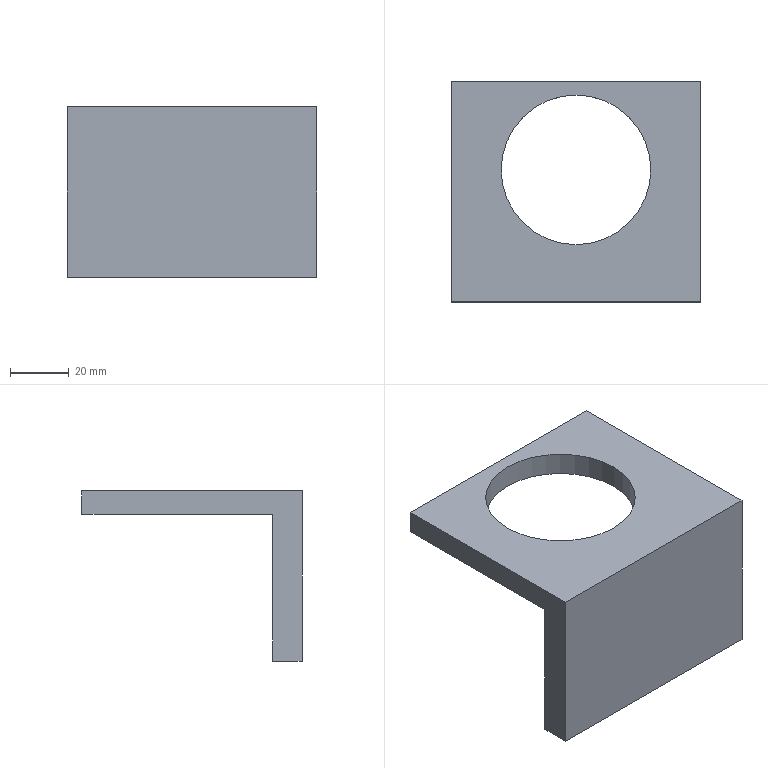Part | SolidWorks | features Extrusion 1, ICE 1 | 1 solid | 10 faces | box 85 x 75 x 58 mm | volume 77157 mm3 | plane 8 | cylinder 2 | commonest cylinder face diameters 51 x2
STEP:
#1=CARTESIAN_POINT('',(-25.5,0.,8.));
#2=VERTEX_POINT('',#1);
#3=CARTESIAN_POINT('',(25.5,0.,8.));
#4=VERTEX_POINT('',#3);
#5=CARTESIAN_POINT('',(0.,0.,8.));
#6=DIRECTION('',(0.,0.,1.));
#7=DIRECTION('',(1.,0.,0.));
#8=AXIS2_PLACEMENT_3D('',#5,#6,#7);
#9=CIRCLE('',#8,25.5);
#10=EDGE_CURVE('',#2,#4,#9,.T.);
#11=ORIENTED_EDGE('',*,*,#10,.T.);
#12=CARTESIAN_POINT('',(25.5,0.,0.));
#13=VERTEX_POINT('',#12);
#14=CARTESIAN_POINT('',(25.5,0.,8.));
#15=DIRECTION('',(0.,0.,-1.));
#16=VECTOR('',#15,1000.);
#17=LINE('',#14,#16);
#18=EDGE_CURVE('',#4,#13,#17,.T.);
#19=ORIENTED_EDGE('',*,*,#18,.T.);
#20=CARTESIAN_POINT('',(-25.5,0.,0.));
#21=VERTEX_POINT('',#20);
#22=CARTESIAN_POINT('',(0.,0.,0.));
#23=DIRECTION('',(0.,0.,1.));
#24=DIRECTION('',(1.,0.,0.));
#25=AXIS2_PLACEMENT_3D('',#22,#23,#24);
#26=CIRCLE('',#25,25.5);
#27=EDGE_CURVE('',#21,#13,#26,.T.);
#28=ORIENTED_EDGE('',*,*,#27,.F.);
#29=CARTESIAN_POINT('',(-25.5,0.,8.));
#30=DIRECTION('',(0.,0.,-1.));
#31=VECTOR('',#30,1000.);
#32=LINE('',#29,#31);
#33=EDGE_CURVE('',#2,#21,#32,.T.);
#34=ORIENTED_EDGE('',*,*,#33,.F.);
#35=EDGE_LOOP('',(#11,#19,#28,#34));
#36=FACE_OUTER_BOUND('',#35,.T.);
#37=CARTESIAN_POINT('',(0.,0.,8.));
#38=DIRECTION('',(0.,0.,-1.));
#39=DIRECTION('',(-1.,0.,0.));
#40=AXIS2_PLACEMENT_3D('',#37,#38,#39);
#41=CYLINDRICAL_SURFACE('',#40,25.5);
#42=ADVANCED_FACE('',(#36),#41,.F.);
#43=CARTESIAN_POINT('',(42.5,-45.,8.));
#44=VERTEX_POINT('',#43);
#45=CARTESIAN_POINT('',(42.5,30.,8.));
#46=VERTEX_POINT('',#45);
#47=CARTESIAN_POINT('',(42.5,-45.,8.));
#48=DIRECTION('',(0.,1.,0.));
#49=VECTOR('',#48,1000.);
#50=LINE('',#47,#49);
#51=EDGE_CURVE('',#44,#46,#50,.T.);
#52=ORIENTED_EDGE('',*,*,#51,.T.);
#53=CARTESIAN_POINT('',(-42.5,30.,8.));
#54=VERTEX_POINT('',#53);
#55=CARTESIAN_POINT('',(-42.5,30.,8.));
#56=DIRECTION('',(-1.,0.,0.));
#57=VECTOR('',#56,1000.);
#58=LINE('',#55,#57);
#59=EDGE_CURVE('',#46,#54,#58,.T.);
#60=ORIENTED_EDGE('',*,*,#59,.T.);
#61=CARTESIAN_POINT('',(-42.5,-45.,8.));
#62=VERTEX_POINT('',#61);
#63=CARTESIAN_POINT('',(-42.5,-45.,8.));
#64=DIRECTION('',(0.,-1.,0.));
#65=VECTOR('',#64,1000.);
#66=LINE('',#63,#65);
#67=EDGE_CURVE('',#54,#62,#66,.T.);
#68=ORIENTED_EDGE('',*,*,#67,.T.);
#69=CARTESIAN_POINT('',(-42.5,-45.,8.));
#70=DIRECTION('',(1.,0.,0.));
#71=VECTOR('',#70,1000.);
#72=LINE('',#69,#71);
#73=EDGE_CURVE('',#62,#44,#72,.T.);
#74=ORIENTED_EDGE('',*,*,#73,.T.);
#75=EDGE_LOOP('',(#52,#60,#68,#74));
#76=FACE_OUTER_BOUND('',#75,.T.);
#77=ORIENTED_EDGE('',*,*,#10,.F.);
#78=CARTESIAN_POINT('',(0.,0.,8.));
#79=DIRECTION('',(0.,0.,1.));
#80=DIRECTION('',(1.,0.,0.));
#81=AXIS2_PLACEMENT_3D('',#78,#79,#80);
#82=CIRCLE('',#81,25.5);
#83=EDGE_CURVE('',#4,#2,#82,.T.);
#84=ORIENTED_EDGE('',*,*,#83,.F.);
#85=EDGE_LOOP('',(#77,#84));
#86=FACE_BOUND('',#85,.T.);
#87=CARTESIAN_POINT('',(0.,0.,8.));
#88=DIRECTION('',(0.,0.,-1.));
#89=DIRECTION('',(-1.,0.,0.));
#90=AXIS2_PLACEMENT_3D('',#87,#88,#89);
#91=PLANE('',#90);
#92=ADVANCED_FACE('',(#76,#86),#91,.F.);
#93=CARTESIAN_POINT('',(-42.5,-35.,0.));
#94=VERTEX_POINT('',#93);
#95=CARTESIAN_POINT('',(42.5,-35.,0.));
#96=VERTEX_POINT('',#95);
#97=CARTESIAN_POINT('',(42.5,-35.,0.));
#98=DIRECTION('',(1.,0.,0.));
#99=VECTOR('',#98,1000.);
#100=LINE('',#97,#99);
#101=EDGE_CURVE('',#94,#96,#100,.T.);
#102=ORIENTED_EDGE('',*,*,#101,.F.);
#103=CARTESIAN_POINT('',(-42.5,30.,0.));
#104=VERTEX_POINT('',#103);
#105=CARTESIAN_POINT('',(-42.5,-45.,0.));
#106=DIRECTION('',(0.,-1.,0.));
#107=VECTOR('',#106,1000.);
#108=LINE('',#105,#107);
#109=EDGE_CURVE('',#104,#94,#108,.T.);
#110=ORIENTED_EDGE('',*,*,#109,.F.);
#111=CARTESIAN_POINT('',(42.5,30.,0.));
#112=VERTEX_POINT('',#111);
#113=CARTESIAN_POINT('',(-42.5,30.,0.));
#114=DIRECTION('',(-1.,0.,0.));
#115=VECTOR('',#114,1000.);
#116=LINE('',#113,#115);
#117=EDGE_CURVE('',#112,#104,#116,.T.);
#118=ORIENTED_EDGE('',*,*,#117,.F.);
#119=CARTESIAN_POINT('',(42.5,-45.,0.));
#120=DIRECTION('',(0.,1.,0.));
#121=VECTOR('',#120,1000.);
#122=LINE('',#119,#121);
#123=EDGE_CURVE('',#96,#112,#122,.T.);
#124=ORIENTED_EDGE('',*,*,#123,.F.);
#125=EDGE_LOOP('',(#102,#110,#118,#124));
#126=FACE_OUTER_BOUND('',#125,.T.);
#127=ORIENTED_EDGE('',*,*,#27,.T.);
#128=CARTESIAN_POINT('',(0.,0.,0.));
#129=DIRECTION('',(0.,0.,1.));
#130=DIRECTION('',(1.,0.,0.));
#131=AXIS2_PLACEMENT_3D('',#128,#129,#130);
#132=CIRCLE('',#131,25.5);
#133=EDGE_CURVE('',#13,#21,#132,.T.);
#134=ORIENTED_EDGE('',*,*,#133,.T.);
#135=EDGE_LOOP('',(#127,#134));
#136=FACE_BOUND('',#135,.T.);
#137=CARTESIAN_POINT('',(0.,0.,0.));
#138=DIRECTION('',(0.,0.,-1.));
#139=DIRECTION('',(-1.,0.,0.));
#140=AXIS2_PLACEMENT_3D('',#137,#138,#139);
#141=PLANE('',#140);
#142=ADVANCED_FACE('',(#126,#136),#141,.T.);
#143=CARTESIAN_POINT('',(42.5,-45.,-50.));
#144=VERTEX_POINT('',#143);
#145=CARTESIAN_POINT('',(42.5,-45.,8.));
#146=DIRECTION('',(0.,0.,-1.));
#147=VECTOR('',#146,1000.);
#148=LINE('',#145,#147);
#149=EDGE_CURVE('',#44,#144,#148,.T.);
#150=ORIENTED_EDGE('',*,*,#149,.T.);
#151=CARTESIAN_POINT('',(42.5,-35.,-50.));
#152=VERTEX_POINT('',#151);
#153=CARTESIAN_POINT('',(42.5,-45.,-50.));
#154=DIRECTION('',(0.,-1.,0.));
#155=VECTOR('',#154,1000.);
#156=LINE('',#153,#155);
#157=EDGE_CURVE('',#152,#144,#156,.T.);
#158=ORIENTED_EDGE('',*,*,#157,.F.);
#159=CARTESIAN_POINT('',(42.5,-35.,-50.));
#160=DIRECTION('',(0.,0.,1.));
#161=VECTOR('',#160,1000.);
#162=LINE('',#159,#161);
#163=EDGE_CURVE('',#152,#96,#162,.T.);
#164=ORIENTED_EDGE('',*,*,#163,.T.);
#165=ORIENTED_EDGE('',*,*,#123,.T.);
#166=CARTESIAN_POINT('',(42.5,30.,8.));
#167=DIRECTION('',(0.,0.,-1.));
#168=VECTOR('',#167,1000.);
#169=LINE('',#166,#168);
#170=EDGE_CURVE('',#46,#112,#169,.T.);
#171=ORIENTED_EDGE('',*,*,#170,.F.);
#172=ORIENTED_EDGE('',*,*,#51,.F.);
#173=EDGE_LOOP('',(#150,#158,#164,#165,#171,#172));
#174=FACE_OUTER_BOUND('',#173,.T.);
#175=CARTESIAN_POINT('',(42.5,-45.,8.));
#176=DIRECTION('',(-1.,0.,0.));
#177=DIRECTION('',(0.,0.,1.));
#178=AXIS2_PLACEMENT_3D('',#175,#176,#177);
#179=PLANE('',#178);
#180=ADVANCED_FACE('',(#174),#179,.F.);
#181=ORIENTED_EDGE('',*,*,#117,.T.);
#182=CARTESIAN_POINT('',(-42.5,30.,8.));
#183=DIRECTION('',(0.,0.,-1.));
#184=VECTOR('',#183,1000.);
#185=LINE('',#182,#184);
#186=EDGE_CURVE('',#54,#104,#185,.T.);
#187=ORIENTED_EDGE('',*,*,#186,.F.);
#188=ORIENTED_EDGE('',*,*,#59,.F.);
#189=ORIENTED_EDGE('',*,*,#170,.T.);
#190=EDGE_LOOP('',(#181,#187,#188,#189));
#191=FACE_OUTER_BOUND('',#190,.T.);
#192=CARTESIAN_POINT('',(-42.5,30.,8.));
#193=DIRECTION('',(0.,-1.,0.));
#194=DIRECTION('',(0.,0.,-1.));
#195=AXIS2_PLACEMENT_3D('',#192,#193,#194);
#196=PLANE('',#195);
#197=ADVANCED_FACE('',(#191),#196,.F.);
#198=ORIENTED_EDGE('',*,*,#109,.T.);
#199=CARTESIAN_POINT('',(-42.5,-35.,-50.));
#200=VERTEX_POINT('',#199);
#201=CARTESIAN_POINT('',(-42.5,-35.,-50.));
#202=DIRECTION('',(0.,0.,1.));
#203=VECTOR('',#202,1000.);
#204=LINE('',#201,#203);
#205=EDGE_CURVE('',#200,#94,#204,.T.);
#206=ORIENTED_EDGE('',*,*,#205,.F.);
#207=CARTESIAN_POINT('',(-42.5,-45.,-50.));
#208=VERTEX_POINT('',#207);
#209=CARTESIAN_POINT('',(-42.5,-45.,-50.));
#210=DIRECTION('',(0.,1.,0.));
#211=VECTOR('',#210,1000.);
#212=LINE('',#209,#211);
#213=EDGE_CURVE('',#208,#200,#212,.T.);
#214=ORIENTED_EDGE('',*,*,#213,.F.);
#215=CARTESIAN_POINT('',(-42.5,-45.,8.));
#216=DIRECTION('',(0.,0.,-1.));
#217=VECTOR('',#216,1000.);
#218=LINE('',#215,#217);
#219=EDGE_CURVE('',#62,#208,#218,.T.);
#220=ORIENTED_EDGE('',*,*,#219,.F.);
#221=ORIENTED_EDGE('',*,*,#67,.F.);
#222=ORIENTED_EDGE('',*,*,#186,.T.);
#223=EDGE_LOOP('',(#198,#206,#214,#220,#221,#222));
#224=FACE_OUTER_BOUND('',#223,.T.);
#225=CARTESIAN_POINT('',(-42.5,-45.,8.));
#226=DIRECTION('',(1.,0.,0.));
#227=DIRECTION('',(0.,0.,-1.));
#228=AXIS2_PLACEMENT_3D('',#225,#226,#227);
#229=PLANE('',#228);
#230=ADVANCED_FACE('',(#224),#229,.F.);
#231=ORIENTED_EDGE('',*,*,#219,.T.);
#232=CARTESIAN_POINT('',(42.5,-45.,-50.));
#233=DIRECTION('',(-1.,0.,0.));
#234=VECTOR('',#233,1000.);
#235=LINE('',#232,#234);
#236=EDGE_CURVE('',#144,#208,#235,.T.);
#237=ORIENTED_EDGE('',*,*,#236,.F.);
#238=ORIENTED_EDGE('',*,*,#149,.F.);
#239=ORIENTED_EDGE('',*,*,#73,.F.);
#240=EDGE_LOOP('',(#231,#237,#238,#239));
#241=FACE_OUTER_BOUND('',#240,.T.);
#242=CARTESIAN_POINT('',(-42.5,-45.,8.));
#243=DIRECTION('',(0.,1.,0.));
#244=DIRECTION('',(0.,0.,1.));
#245=AXIS2_PLACEMENT_3D('',#242,#243,#244);
#246=PLANE('',#245);
#247=ADVANCED_FACE('',(#241),#246,.F.);
#248=ORIENTED_EDGE('',*,*,#18,.F.);
#249=ORIENTED_EDGE('',*,*,#83,.T.);
#250=ORIENTED_EDGE('',*,*,#33,.T.);
#251=ORIENTED_EDGE('',*,*,#133,.F.);
#252=EDGE_LOOP('',(#248,#249,#250,#251));
#253=FACE_OUTER_BOUND('',#252,.T.);
#254=CARTESIAN_POINT('',(0.,0.,8.));
#255=DIRECTION('',(0.,0.,-1.));
#256=DIRECTION('',(-1.,0.,0.));
#257=AXIS2_PLACEMENT_3D('',#254,#255,#256);
#258=CYLINDRICAL_SURFACE('',#257,25.5);
#259=ADVANCED_FACE('',(#253),#258,.F.);
#260=ORIENTED_EDGE('',*,*,#101,.T.);
#261=ORIENTED_EDGE('',*,*,#163,.F.);
#262=CARTESIAN_POINT('',(42.5,-35.,-50.));
#263=DIRECTION('',(1.,0.,0.));
#264=VECTOR('',#263,1000.);
#265=LINE('',#262,#264);
#266=EDGE_CURVE('',#200,#152,#265,.T.);
#267=ORIENTED_EDGE('',*,*,#266,.F.);
#268=ORIENTED_EDGE('',*,*,#205,.T.);
#269=EDGE_LOOP('',(#260,#261,#267,#268));
#270=FACE_OUTER_BOUND('',#269,.T.);
#271=CARTESIAN_POINT('',(42.5,-35.,-50.));
#272=DIRECTION('',(0.,-1.,0.));
#273=DIRECTION('',(0.,0.,-1.));
#274=AXIS2_PLACEMENT_3D('',#271,#272,#273);
#275=PLANE('',#274);
#276=ADVANCED_FACE('',(#270),#275,.F.);
#277=ORIENTED_EDGE('',*,*,#157,.T.);
#278=ORIENTED_EDGE('',*,*,#236,.T.);
#279=ORIENTED_EDGE('',*,*,#213,.T.);
#280=ORIENTED_EDGE('',*,*,#266,.T.);
#281=EDGE_LOOP('',(#277,#278,#279,#280));
#282=FACE_OUTER_BOUND('',#281,.T.);
#283=CARTESIAN_POINT('',(0.,0.,-50.));
#284=DIRECTION('',(0.,0.,1.));
#285=DIRECTION('',(1.,0.,0.));
#286=AXIS2_PLACEMENT_3D('',#283,#284,#285);
#287=PLANE('',#286);
#288=ADVANCED_FACE('',(#282),#287,.F.);
#289=CLOSED_SHELL('',(#42,#92,#142,#180,#197,#230,#247,#259,#276,#288));
#290=MANIFOLD_SOLID_BREP('',#289);
#291=CARTESIAN_POINT('',(0.,0.,0.));
#292=DIRECTION('',(0.,0.,1.));
#293=DIRECTION('',(1.,0.,0.));
#294=AXIS2_PLACEMENT_3D('',#291,#292,#293);
#295=(LENGTH_UNIT()NAMED_UNIT(*)SI_UNIT(.MILLI.,.METRE.));
#296=UNCERTAINTY_MEASURE_WITH_UNIT(LENGTH_MEASURE(0.00001),#295,'','');
#297=(NAMED_UNIT(*)PLANE_ANGLE_UNIT()SI_UNIT($,.RADIAN.));
#298=(NAMED_UNIT(*)SI_UNIT($,.STERADIAN.)SOLID_ANGLE_UNIT());
#299=(GEOMETRIC_REPRESENTATION_CONTEXT(3)GLOBAL_UNCERTAINTY_ASSIGNED_CONTEXT((#296))GLOBAL_UNIT_ASSIGNED_CONTEXT((#295,#297,#298))REPRESENTATION_CONTEXT('',''));
#300=ADVANCED_BREP_SHAPE_REPRESENTATION('',(#290,#294),#299);